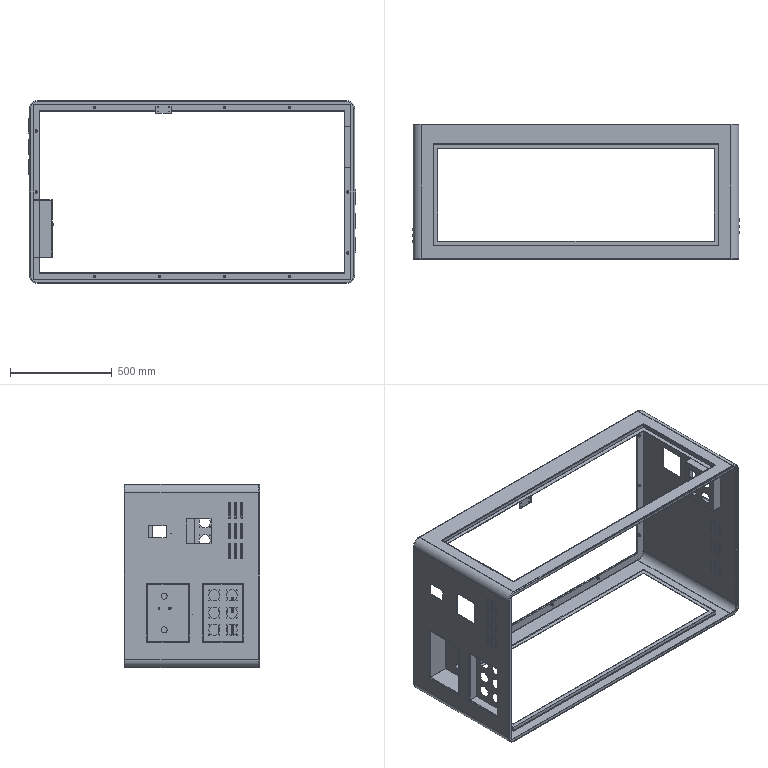Part | STEP file | B-002 | 1 solid | 646 faces | box 1610 x 665 x 900 mm | volume 5357504 mm3 | cylinder 356 | plane 206 | sphere 72 | torus 12 | commonest cylinder face diameters 3.3 x92 7 x72 10 x66 5 x28 12 x28 6 x20